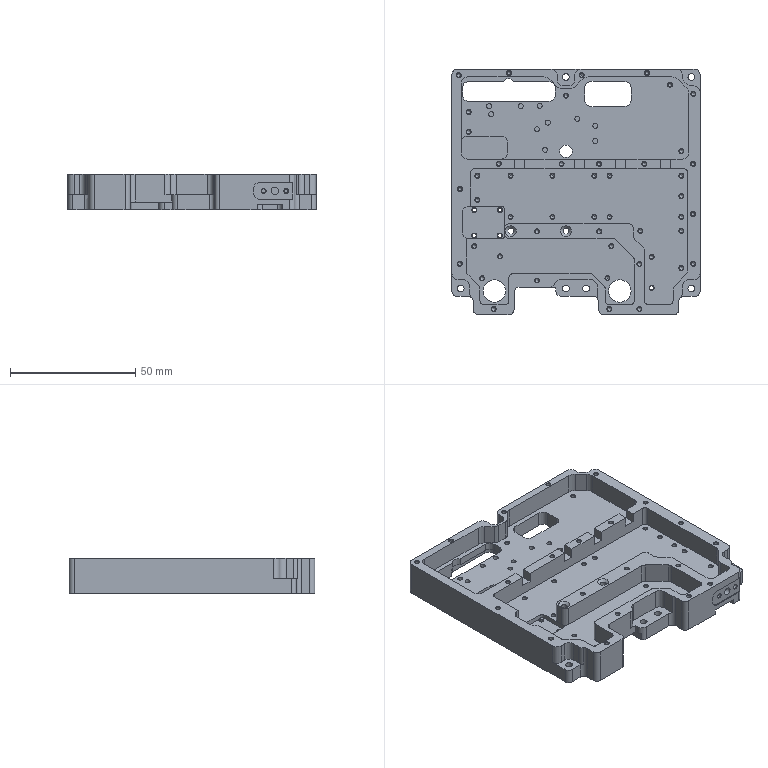Part | STEP file | Driver amplifier module cavity | 1 solid | 426 faces | box 99 x 98 x 14 mm | volume 63567 mm3 | cylinder 178 | plane 137 | cone 111 | commonest cylinder face diameters 1.6 x55 5 x55 4 x26 2 x12 3 x10 2.7 x6